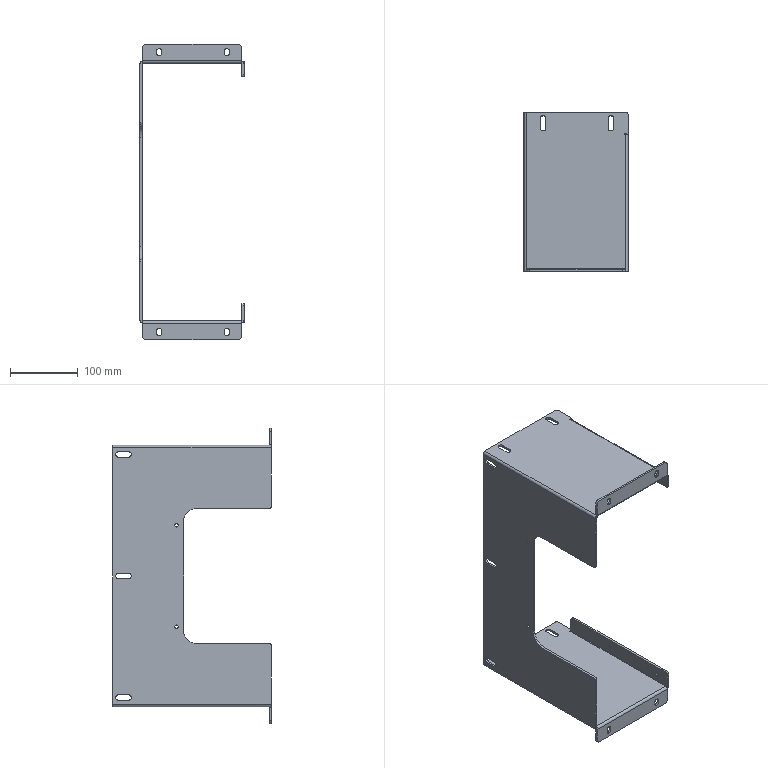Part | SolidWorks | features Fillet 4, ICE 4, EdgeFlange 3, HoleWzd 2, Cut 1, FlatPattern 1, SMBaseFlange 1, SheetMetal 1 | 1 solid | 144 faces | box 154 x 235 x 437 mm | volume 449596 mm3 | plane 80 | cylinder 64 | commonest cylinder face diameters 8 x26 5 x12 6 x8 1 x6 7 x6 10 x4